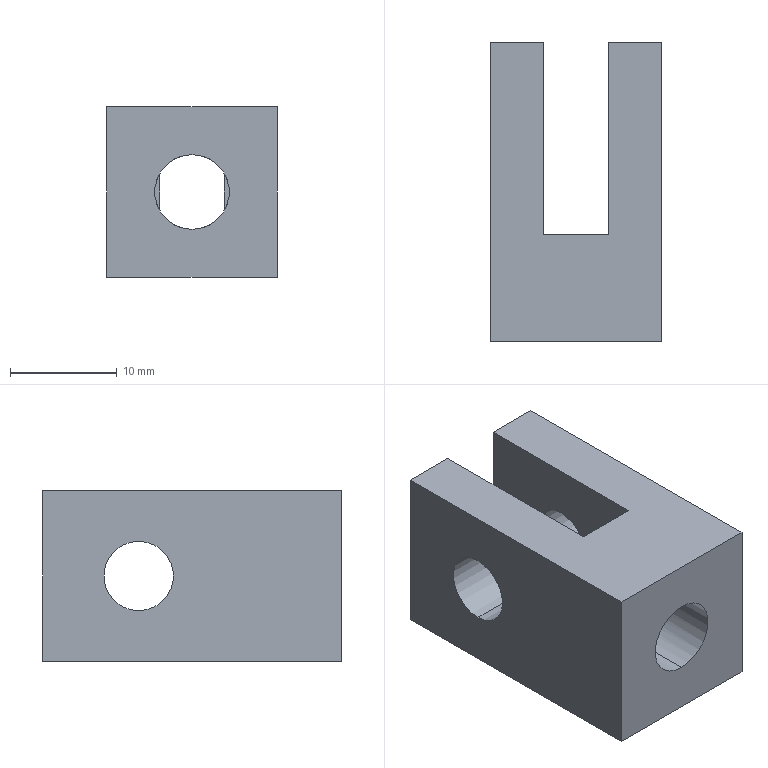Part | STEP file | BU-C05-1 | 1 solid | 19 faces | box 16 x 28 x 16 mm | volume 4723 mm3 | plane 13 | cylinder 6 | commonest cylinder face diameters 6.5 x4 7 x2
STEP:
#1=CARTESIAN_POINT('',(0.,0.,0.));
#2=DIRECTION('',(0.,0.,1.));
#3=DIRECTION('',(1.,0.,0.));
#4=AXIS2_PLACEMENT_3D('',#1,#2,#3);
#5=CARTESIAN_POINT('',(-3.,19.,11.25));
#6=VERTEX_POINT('',#5);
#7=CARTESIAN_POINT('',(-8.,19.,11.25));
#8=VERTEX_POINT('',#7);
#9=CARTESIAN_POINT('',(-8.,19.,11.25));
#10=DIRECTION('',(-1.,0.,0.));
#11=VECTOR('',#10,1.);
#12=LINE('',#9,#11);
#13=CARTESIAN_POINT('',(-8.,19.,8.));
#14=DIRECTION('',(-1.,0.,0.));
#15=DIRECTION('',(0.,0.,1.));
#16=AXIS2_PLACEMENT_3D('',#13,#14,#15);
#17=CYLINDRICAL_SURFACE('',#16,3.25);
#18=CARTESIAN_POINT('',(6.283,0.));
#19=DIRECTION('',(0.,1.));
#20=VECTOR('',#19,1.);
#21=LINE('',#18,#20);
#22=(GEOMETRIC_REPRESENTATION_CONTEXT(2)PARAMETRIC_REPRESENTATION_CONTEXT()REPRESENTATION_CONTEXT('',''));
#23=DEFINITIONAL_REPRESENTATION('',(#21),#22);
#24=PCURVE('',#17,#23);
#25=CARTESIAN_POINT('',(-8.,19.,8.));
#26=DIRECTION('',(-1.,0.,0.));
#27=DIRECTION('',(0.,0.,1.));
#28=AXIS2_PLACEMENT_3D('',#25,#26,#27);
#29=CYLINDRICAL_SURFACE('',#28,3.25);
#30=CARTESIAN_POINT('',(0.,0.));
#31=DIRECTION('',(0.,1.));
#32=VECTOR('',#31,1.);
#33=LINE('',#30,#32);
#34=(GEOMETRIC_REPRESENTATION_CONTEXT(2)PARAMETRIC_REPRESENTATION_CONTEXT()REPRESENTATION_CONTEXT('',''));
#35=DEFINITIONAL_REPRESENTATION('',(#33),#34);
#36=PCURVE('',#29,#35);
#37=SURFACE_CURVE('',#12,(#24,#36),.PCURVE_S1.);
#38=EDGE_CURVE('',#6,#8,#37,.T.);
#39=ORIENTED_EDGE('',*,*,#38,.T.);
#40=CARTESIAN_POINT('',(-8.,19.,4.75));
#41=VERTEX_POINT('',#40);
#42=CARTESIAN_POINT('',(-8.,19.,8.));
#43=DIRECTION('',(-1.,0.,0.));
#44=DIRECTION('',(0.,0.,1.));
#45=AXIS2_PLACEMENT_3D('',#42,#43,#44);
#46=CIRCLE('',#45,3.25);
#47=CARTESIAN_POINT('',(0.,0.));
#48=DIRECTION('',(1.,0.));
#49=VECTOR('',#48,1.);
#50=LINE('',#47,#49);
#51=(GEOMETRIC_REPRESENTATION_CONTEXT(2)PARAMETRIC_REPRESENTATION_CONTEXT()REPRESENTATION_CONTEXT('',''));
#52=DEFINITIONAL_REPRESENTATION('',(#50),#51);
#53=PCURVE('',#17,#52);
#54=CARTESIAN_POINT('',(-8.,0.,16.));
#55=DIRECTION('',(1.,0.,0.));
#56=DIRECTION('',(0.,0.,-1.));
#57=AXIS2_PLACEMENT_3D('',#54,#55,#56);
#58=PLANE('',#57);
#59=CARTESIAN_POINT('',(4.75,19.));
#60=CARTESIAN_POINT('',(4.75,24.629));
#61=CARTESIAN_POINT('',(9.625,21.815));
#62=CARTESIAN_POINT('',(14.5,19.));
#63=CARTESIAN_POINT('',(9.625,16.185));
#64=CARTESIAN_POINT('',(4.75,13.371));
#65=CARTESIAN_POINT('',(4.75,19.));
#66=(BOUNDED_CURVE()B_SPLINE_CURVE(2,(#59,#60,#61,#62,#63,#64,#65),.UNSPECIFIED.,.T.,.F.)B_SPLINE_CURVE_WITH_KNOTS((1,2,2,2,2,1),(-2.094,0.,2.094,4.189,6.283,8.378),.UNSPECIFIED.)CURVE()GEOMETRIC_REPRESENTATION_ITEM()RATIONAL_B_SPLINE_CURVE((1.,0.5,1.,0.5,1.,0.5,1.))REPRESENTATION_ITEM(''));
#67=(GEOMETRIC_REPRESENTATION_CONTEXT(2)PARAMETRIC_REPRESENTATION_CONTEXT()REPRESENTATION_CONTEXT('',''));
#68=DEFINITIONAL_REPRESENTATION('',(#66),#67);
#69=PCURVE('',#58,#68);
#70=SURFACE_CURVE('',#46,(#53,#69),.PCURVE_S1.);
#71=EDGE_CURVE('',#41,#8,#70,.T.);
#72=ORIENTED_EDGE('',*,*,#71,.F.);
#73=CARTESIAN_POINT('',(-3.,19.,4.75));
#74=VERTEX_POINT('',#73);
#75=CARTESIAN_POINT('',(-8.,19.,4.75));
#76=DIRECTION('',(-1.,0.,0.));
#77=VECTOR('',#76,1.);
#78=LINE('',#75,#77);
#79=CARTESIAN_POINT('',(3.142,0.));
#80=DIRECTION('',(0.,1.));
#81=VECTOR('',#80,1.);
#82=LINE('',#79,#81);
#83=(GEOMETRIC_REPRESENTATION_CONTEXT(2)PARAMETRIC_REPRESENTATION_CONTEXT()REPRESENTATION_CONTEXT('',''));
#84=DEFINITIONAL_REPRESENTATION('',(#82),#83);
#85=PCURVE('',#17,#84);
#86=CARTESIAN_POINT('',(3.142,0.));
#87=DIRECTION('',(0.,1.));
#88=VECTOR('',#87,1.);
#89=LINE('',#86,#88);
#90=(GEOMETRIC_REPRESENTATION_CONTEXT(2)PARAMETRIC_REPRESENTATION_CONTEXT()REPRESENTATION_CONTEXT('',''));
#91=DEFINITIONAL_REPRESENTATION('',(#89),#90);
#92=PCURVE('',#29,#91);
#93=SURFACE_CURVE('',#78,(#85,#92),.PCURVE_S1.);
#94=EDGE_CURVE('',#74,#41,#93,.T.);
#95=ORIENTED_EDGE('',*,*,#94,.F.);
#96=CARTESIAN_POINT('',(-3.,19.,8.));
#97=DIRECTION('',(-1.,0.,0.));
#98=DIRECTION('',(0.,0.,1.));
#99=AXIS2_PLACEMENT_3D('',#96,#97,#98);
#100=CIRCLE('',#99,3.25);
#101=CARTESIAN_POINT('',(0.,-5.));
#102=DIRECTION('',(1.,0.));
#103=VECTOR('',#102,1.);
#104=LINE('',#101,#103);
#105=(GEOMETRIC_REPRESENTATION_CONTEXT(2)PARAMETRIC_REPRESENTATION_CONTEXT()REPRESENTATION_CONTEXT('',''));
#106=DEFINITIONAL_REPRESENTATION('',(#104),#105);
#107=PCURVE('',#17,#106);
#108=CARTESIAN_POINT('',(-3.,10.,16.));
#109=DIRECTION('',(-1.,0.,0.));
#110=DIRECTION('',(0.,0.,1.));
#111=AXIS2_PLACEMENT_3D('',#108,#109,#110);
#112=PLANE('',#111);
#113=CARTESIAN_POINT('',(-8.,9.));
#114=DIRECTION('',(1.,0.));
#115=AXIS2_PLACEMENT_2D('',#113,#114);
#116=CIRCLE('',#115,3.25);
#117=(GEOMETRIC_REPRESENTATION_CONTEXT(2)PARAMETRIC_REPRESENTATION_CONTEXT()REPRESENTATION_CONTEXT('',''));
#118=DEFINITIONAL_REPRESENTATION('',(#116),#117);
#119=PCURVE('',#112,#118);
#120=SURFACE_CURVE('',#100,(#107,#119),.PCURVE_S1.);
#121=EDGE_CURVE('',#74,#6,#120,.T.);
#122=ORIENTED_EDGE('',*,*,#121,.T.);
#123=EDGE_LOOP('',(#39,#72,#95,#122));
#124=FACE_BOUND('',#123,.F.);
#125=ADVANCED_FACE('',(#124),#17,.F.);
#126=CARTESIAN_POINT('',(8.,19.,11.25));
#127=VERTEX_POINT('',#126);
#128=CARTESIAN_POINT('',(3.,19.,11.25));
#129=VERTEX_POINT('',#128);
#130=CARTESIAN_POINT('',(-8.,19.,11.25));
#131=DIRECTION('',(-1.,0.,0.));
#132=VECTOR('',#131,1.);
#133=LINE('',#130,#132);
#134=CARTESIAN_POINT('',(-8.,19.,8.));
#135=DIRECTION('',(-1.,0.,0.));
#136=DIRECTION('',(0.,0.,1.));
#137=AXIS2_PLACEMENT_3D('',#134,#135,#136);
#138=CYLINDRICAL_SURFACE('',#137,3.25);
#139=CARTESIAN_POINT('',(6.283,0.));
#140=DIRECTION('',(0.,1.));
#141=VECTOR('',#140,1.);
#142=LINE('',#139,#141);
#143=(GEOMETRIC_REPRESENTATION_CONTEXT(2)PARAMETRIC_REPRESENTATION_CONTEXT()REPRESENTATION_CONTEXT('',''));
#144=DEFINITIONAL_REPRESENTATION('',(#142),#143);
#145=PCURVE('',#138,#144);
#146=CARTESIAN_POINT('',(-8.,19.,8.));
#147=DIRECTION('',(-1.,0.,0.));
#148=DIRECTION('',(0.,0.,1.));
#149=AXIS2_PLACEMENT_3D('',#146,#147,#148);
#150=CYLINDRICAL_SURFACE('',#149,3.25);
#151=CARTESIAN_POINT('',(0.,0.));
#152=DIRECTION('',(0.,1.));
#153=VECTOR('',#152,1.);
#154=LINE('',#151,#153);
#155=(GEOMETRIC_REPRESENTATION_CONTEXT(2)PARAMETRIC_REPRESENTATION_CONTEXT()REPRESENTATION_CONTEXT('',''));
#156=DEFINITIONAL_REPRESENTATION('',(#154),#155);
#157=PCURVE('',#150,#156);
#158=SURFACE_CURVE('',#133,(#145,#157),.PCURVE_S1.);
#159=EDGE_CURVE('',#127,#129,#158,.T.);
#160=ORIENTED_EDGE('',*,*,#159,.T.);
#161=CARTESIAN_POINT('',(3.,19.,4.75));
#162=VERTEX_POINT('',#161);
#163=CARTESIAN_POINT('',(3.,19.,8.));
#164=DIRECTION('',(1.,0.,0.));
#165=DIRECTION('',(0.,0.,-1.));
#166=AXIS2_PLACEMENT_3D('',#163,#164,#165);
#167=CIRCLE('',#166,3.25);
#168=CARTESIAN_POINT('',(9.425,-11.));
#169=DIRECTION('',(-1.,0.));
#170=VECTOR('',#169,1.);
#171=LINE('',#168,#170);
#172=(GEOMETRIC_REPRESENTATION_CONTEXT(2)PARAMETRIC_REPRESENTATION_CONTEXT()REPRESENTATION_CONTEXT('',''));
#173=DEFINITIONAL_REPRESENTATION('',(#171),#172);
#174=PCURVE('',#138,#173);
#175=CARTESIAN_POINT('',(3.,10.,16.));
#176=DIRECTION('',(1.,0.,0.));
#177=DIRECTION('',(0.,0.,-1.));
#178=AXIS2_PLACEMENT_3D('',#175,#176,#177);
#179=PLANE('',#178);
#180=CARTESIAN_POINT('',(8.,9.));
#181=DIRECTION('',(1.,0.));
#182=AXIS2_PLACEMENT_2D('',#180,#181);
#183=CIRCLE('',#182,3.25);
#184=(GEOMETRIC_REPRESENTATION_CONTEXT(2)PARAMETRIC_REPRESENTATION_CONTEXT()REPRESENTATION_CONTEXT('',''));
#185=DEFINITIONAL_REPRESENTATION('',(#183),#184);
#186=PCURVE('',#179,#185);
#187=SURFACE_CURVE('',#167,(#174,#186),.PCURVE_S1.);
#188=EDGE_CURVE('',#129,#162,#187,.T.);
#189=ORIENTED_EDGE('',*,*,#188,.T.);
#190=CARTESIAN_POINT('',(8.,19.,4.75));
#191=VERTEX_POINT('',#190);
#192=CARTESIAN_POINT('',(-8.,19.,4.75));
#193=DIRECTION('',(-1.,0.,0.));
#194=VECTOR('',#193,1.);
#195=LINE('',#192,#194);
#196=CARTESIAN_POINT('',(3.142,0.));
#197=DIRECTION('',(0.,1.));
#198=VECTOR('',#197,1.);
#199=LINE('',#196,#198);
#200=(GEOMETRIC_REPRESENTATION_CONTEXT(2)PARAMETRIC_REPRESENTATION_CONTEXT()REPRESENTATION_CONTEXT('',''));
#201=DEFINITIONAL_REPRESENTATION('',(#199),#200);
#202=PCURVE('',#138,#201);
#203=CARTESIAN_POINT('',(3.142,0.));
#204=DIRECTION('',(0.,1.));
#205=VECTOR('',#204,1.);
#206=LINE('',#203,#205);
#207=(GEOMETRIC_REPRESENTATION_CONTEXT(2)PARAMETRIC_REPRESENTATION_CONTEXT()REPRESENTATION_CONTEXT('',''));
#208=DEFINITIONAL_REPRESENTATION('',(#206),#207);
#209=PCURVE('',#150,#208);
#210=SURFACE_CURVE('',#195,(#202,#209),.PCURVE_S1.);
#211=EDGE_CURVE('',#191,#162,#210,.T.);
#212=ORIENTED_EDGE('',*,*,#211,.F.);
#213=CARTESIAN_POINT('',(8.,19.,8.));
#214=DIRECTION('',(-1.,0.,0.));
#215=DIRECTION('',(0.,0.,1.));
#216=AXIS2_PLACEMENT_3D('',#213,#214,#215);
#217=CIRCLE('',#216,3.25);
#218=CARTESIAN_POINT('',(0.,-16.));
#219=DIRECTION('',(1.,0.));
#220=VECTOR('',#219,1.);
#221=LINE('',#218,#220);
#222=(GEOMETRIC_REPRESENTATION_CONTEXT(2)PARAMETRIC_REPRESENTATION_CONTEXT()REPRESENTATION_CONTEXT('',''));
#223=DEFINITIONAL_REPRESENTATION('',(#221),#222);
#224=PCURVE('',#138,#223);
#225=CARTESIAN_POINT('',(8.,0.,16.));
#226=DIRECTION('',(-1.,0.,0.));
#227=DIRECTION('',(0.,0.,1.));
#228=AXIS2_PLACEMENT_3D('',#225,#226,#227);
#229=PLANE('',#228);
#230=CARTESIAN_POINT('',(-8.,19.));
#231=DIRECTION('',(1.,0.));
#232=AXIS2_PLACEMENT_2D('',#230,#231);
#233=CIRCLE('',#232,3.25);
#234=(GEOMETRIC_REPRESENTATION_CONTEXT(2)PARAMETRIC_REPRESENTATION_CONTEXT()REPRESENTATION_CONTEXT('',''));
#235=DEFINITIONAL_REPRESENTATION('',(#233),#234);
#236=PCURVE('',#229,#235);
#237=SURFACE_CURVE('',#217,(#224,#236),.PCURVE_S1.);
#238=EDGE_CURVE('',#191,#127,#237,.T.);
#239=ORIENTED_EDGE('',*,*,#238,.T.);
#240=EDGE_LOOP('',(#160,#189,#212,#239));
#241=FACE_BOUND('',#240,.F.);
#242=ADVANCED_FACE('',(#241),#138,.F.);
#243=CARTESIAN_POINT('',(-3.,10.,6.197));
#244=VERTEX_POINT('',#243);
#245=CARTESIAN_POINT('',(-3.,10.,9.803));
#246=VERTEX_POINT('',#245);
#247=CARTESIAN_POINT('',(0.,10.,8.));
#248=DIRECTION('',(0.,1.,0.));
#249=DIRECTION('',(0.,0.,-1.));
#250=AXIS2_PLACEMENT_3D('',#247,#248,#249);
#251=CIRCLE('',#250,3.5);
#252=CARTESIAN_POINT('',(0.,0.,8.));
#253=DIRECTION('',(0.,-1.,0.));
#254=DIRECTION('',(0.,0.,-1.));
#255=AXIS2_PLACEMENT_3D('',#252,#253,#254);
#256=CYLINDRICAL_SURFACE('',#255,3.5);
#257=CARTESIAN_POINT('',(6.283,-10.));
#258=DIRECTION('',(-1.,0.));
#259=VECTOR('',#258,1.);
#260=LINE('',#257,#259);
#261=(GEOMETRIC_REPRESENTATION_CONTEXT(2)PARAMETRIC_REPRESENTATION_CONTEXT()REPRESENTATION_CONTEXT('',''));
#262=DEFINITIONAL_REPRESENTATION('',(#260),#261);
#263=PCURVE('',#256,#262);
#264=CARTESIAN_POINT('',(-3.,10.,16.));
#265=DIRECTION('',(0.,-1.,0.));
#266=DIRECTION('',(0.,0.,-1.));
#267=AXIS2_PLACEMENT_3D('',#264,#265,#266);
#268=PLANE('',#267);
#269=CARTESIAN_POINT('',(11.5,3.));
#270=CARTESIAN_POINT('',(11.5,-3.062));
#271=CARTESIAN_POINT('',(6.25,-0.03109));
#272=CARTESIAN_POINT('',(1.,3.));
#273=CARTESIAN_POINT('',(6.25,6.031));
#274=CARTESIAN_POINT('',(11.5,9.062));
#275=CARTESIAN_POINT('',(11.5,3.));
#276=(BOUNDED_CURVE()B_SPLINE_CURVE(2,(#269,#270,#271,#272,#273,#274,#275),.UNSPECIFIED.,.T.,.F.)B_SPLINE_CURVE_WITH_KNOTS((1,2,2,2,2,1),(-2.094,0.,2.094,4.189,6.283,8.378),.UNSPECIFIED.)CURVE()GEOMETRIC_REPRESENTATION_ITEM()RATIONAL_B_SPLINE_CURVE((1.,0.5,1.,0.5,1.,0.5,1.))REPRESENTATION_ITEM(''));
#277=(GEOMETRIC_REPRESENTATION_CONTEXT(2)PARAMETRIC_REPRESENTATION_CONTEXT()REPRESENTATION_CONTEXT('',''));
#278=DEFINITIONAL_REPRESENTATION('',(#276),#277);
#279=PCURVE('',#268,#278);
#280=SURFACE_CURVE('',#251,(#263,#279),.PCURVE_S1.);
#281=EDGE_CURVE('',#244,#246,#280,.T.);
#282=ORIENTED_EDGE('',*,*,#281,.F.);
#283=CARTESIAN_POINT('',(0.,10.,4.5));
#284=VERTEX_POINT('',#283);
#285=CARTESIAN_POINT('',(0.,10.,8.));
#286=DIRECTION('',(0.,1.,0.));
#287=DIRECTION('',(0.,0.,-1.));
#288=AXIS2_PLACEMENT_3D('',#285,#286,#287);
#289=CIRCLE('',#288,3.5);
#290=CARTESIAN_POINT('',(6.283,-10.));
#291=DIRECTION('',(-1.,0.));
#292=VECTOR('',#291,1.);
#293=LINE('',#290,#292);
#294=(GEOMETRIC_REPRESENTATION_CONTEXT(2)PARAMETRIC_REPRESENTATION_CONTEXT()REPRESENTATION_CONTEXT('',''));
#295=DEFINITIONAL_REPRESENTATION('',(#293),#294);
#296=PCURVE('',#256,#295);
#297=CARTESIAN_POINT('',(-3.,10.,16.));
#298=DIRECTION('',(0.,-1.,0.));
#299=DIRECTION('',(0.,0.,-1.));
#300=AXIS2_PLACEMENT_3D('',#297,#298,#299);
#301=PLANE('',#300);
#302=CARTESIAN_POINT('',(11.5,3.));
#303=CARTESIAN_POINT('',(11.5,-3.062));
#304=CARTESIAN_POINT('',(6.25,-0.03109));
#305=CARTESIAN_POINT('',(1.,3.));
#306=CARTESIAN_POINT('',(6.25,6.031));
#307=CARTESIAN_POINT('',(11.5,9.062));
#308=CARTESIAN_POINT('',(11.5,3.));
#309=(BOUNDED_CURVE()B_SPLINE_CURVE(2,(#302,#303,#304,#305,#306,#307,#308),.UNSPECIFIED.,.T.,.F.)B_SPLINE_CURVE_WITH_KNOTS((1,2,2,2,2,1),(-2.094,0.,2.094,4.189,6.283,8.378),.UNSPECIFIED.)CURVE()GEOMETRIC_REPRESENTATION_ITEM()RATIONAL_B_SPLINE_CURVE((1.,0.5,1.,0.5,1.,0.5,1.))REPRESENTATION_ITEM(''));
#310=(GEOMETRIC_REPRESENTATION_CONTEXT(2)PARAMETRIC_REPRESENTATION_CONTEXT()REPRESENTATION_CONTEXT('',''));
#311=DEFINITIONAL_REPRESENTATION('',(#309),#310);
#312=PCURVE('',#301,#311);
#313=SURFACE_CURVE('',#289,(#296,#312),.PCURVE_S1.);
#314=EDGE_CURVE('',#284,#244,#313,.T.);
#315=ORIENTED_EDGE('',*,*,#314,.F.);
#316=CARTESIAN_POINT('',(0.,0.,4.5));
#317=VERTEX_POINT('',#316);
#318=CARTESIAN_POINT('',(0.,0.,4.5));
#319=DIRECTION('',(0.,-1.,0.));
#320=VECTOR('',#319,1.);
#321=LINE('',#318,#320);
#322=CARTESIAN_POINT('',(6.283,0.));
#323=DIRECTION('',(0.,1.));
#324=VECTOR('',#323,1.);
#325=LINE('',#322,#324);
#326=(GEOMETRIC_REPRESENTATION_CONTEXT(2)PARAMETRIC_REPRESENTATION_CONTEXT()REPRESENTATION_CONTEXT('',''));
#327=DEFINITIONAL_REPRESENTATION('',(#325),#326);
#328=PCURVE('',#256,#327);
#329=CARTESIAN_POINT('',(0.,0.,8.));
#330=DIRECTION('',(0.,-1.,0.));
#331=DIRECTION('',(0.,0.,-1.));
#332=AXIS2_PLACEMENT_3D('',#329,#330,#331);
#333=CYLINDRICAL_SURFACE('',#332,3.5);
#334=CARTESIAN_POINT('',(0.,0.));
#335=DIRECTION('',(0.,1.));
#336=VECTOR('',#335,1.);
#337=LINE('',#334,#336);
#338=(GEOMETRIC_REPRESENTATION_CONTEXT(2)PARAMETRIC_REPRESENTATION_CONTEXT()REPRESENTATION_CONTEXT('',''));
#339=DEFINITIONAL_REPRESENTATION('',(#337),#338);
#340=PCURVE('',#333,#339);
#341=SURFACE_CURVE('',#321,(#328,#340),.PCURVE_S1.);
#342=EDGE_CURVE('',#284,#317,#341,.T.);
#343=ORIENTED_EDGE('',*,*,#342,.T.);
#344=CARTESIAN_POINT('',(0.,0.,11.5));
#345=VERTEX_POINT('',#344);
#346=CARTESIAN_POINT('',(0.,0.,8.));
#347=DIRECTION('',(0.,-1.,0.));
#348=DIRECTION('',(0.,0.,-1.));
#349=AXIS2_PLACEMENT_3D('',#346,#347,#348);
#350=CIRCLE('',#349,3.5);
#351=CARTESIAN_POINT('',(0.,0.));
#352=DIRECTION('',(1.,0.));
#353=VECTOR('',#352,1.);
#354=LINE('',#351,#353);
#355=(GEOMETRIC_REPRESENTATION_CONTEXT(2)PARAMETRIC_REPRESENTATION_CONTEXT()REPRESENTATION_CONTEXT('',''));
#356=DEFINITIONAL_REPRESENTATION('',(#354),#355);
#357=PCURVE('',#256,#356);
#358=CARTESIAN_POINT('',(-8.,0.,16.));
#359=DIRECTION('',(0.,1.,0.));
#360=DIRECTION('',(0.,0.,1.));
#361=AXIS2_PLACEMENT_3D('',#358,#359,#360);
#362=PLANE('',#361);
#363=CARTESIAN_POINT('',(-11.5,8.));
#364=CARTESIAN_POINT('',(-11.5,14.062));
#365=CARTESIAN_POINT('',(-6.25,11.031));
#366=CARTESIAN_POINT('',(-1.,8.));
#367=CARTESIAN_POINT('',(-6.25,4.969));
#368=CARTESIAN_POINT('',(-11.5,1.938));
#369=CARTESIAN_POINT('',(-11.5,8.));
#370=(BOUNDED_CURVE()B_SPLINE_CURVE(2,(#363,#364,#365,#366,#367,#368,#369),.UNSPECIFIED.,.T.,.F.)B_SPLINE_CURVE_WITH_KNOTS((1,2,2,2,2,1),(-2.094,0.,2.094,4.189,6.283,8.378),.UNSPECIFIED.)CURVE()GEOMETRIC_REPRESENTATION_ITEM()RATIONAL_B_SPLINE_CURVE((1.,0.5,1.,0.5,1.,0.5,1.))REPRESENTATION_ITEM(''));
#371=(GEOMETRIC_REPRESENTATION_CONTEXT(2)PARAMETRIC_REPRESENTATION_CONTEXT()REPRESENTATION_CONTEXT('',''));
#372=DEFINITIONAL_REPRESENTATION('',(#370),#371);
#373=PCURVE('',#362,#372);
#374=SURFACE_CURVE('',#350,(#357,#373),.PCURVE_S1.);
#375=EDGE_CURVE('',#345,#317,#374,.T.);
#376=ORIENTED_EDGE('',*,*,#375,.F.);
#377=CARTESIAN_POINT('',(0.,10.,11.5));
#378=VERTEX_POINT('',#377);
#379=CARTESIAN_POINT('',(0.,0.,11.5));
#380=DIRECTION('',(0.,-1.,0.));
#381=VECTOR('',#380,1.);
#382=LINE('',#379,#381);
#383=CARTESIAN_POINT('',(3.142,0.));
#384=DIRECTION('',(0.,1.));
#385=VECTOR('',#384,1.);
#386=LINE('',#383,#385);
#387=(GEOMETRIC_REPRESENTATION_CONTEXT(2)PARAMETRIC_REPRESENTATION_CONTEXT()REPRESENTATION_CONTEXT('',''));
#388=DEFINITIONAL_REPRESENTATION('',(#386),#387);
#389=PCURVE('',#256,#388);
#390=CARTESIAN_POINT('',(3.142,0.));
#391=DIRECTION('',(0.,1.));
#392=VECTOR('',#391,1.);
#393=LINE('',#390,#392);
#394=(GEOMETRIC_REPRESENTATION_CONTEXT(2)PARAMETRIC_REPRESENTATION_CONTEXT()REPRESENTATION_CONTEXT('',''));
#395=DEFINITIONAL_REPRESENTATION('',(#393),#394);
#396=PCURVE('',#333,#395);
#397=SURFACE_CURVE('',#382,(#389,#396),.PCURVE_S1.);
#398=EDGE_CURVE('',#378,#345,#397,.T.);
#399=ORIENTED_EDGE('',*,*,#398,.F.);
#400=CARTESIAN_POINT('',(0.,10.,8.));
#401=DIRECTION('',(0.,1.,0.));
#402=DIRECTION('',(0.,0.,-1.));
#403=AXIS2_PLACEMENT_3D('',#400,#401,#402);
#404=CIRCLE('',#403,3.5);
#405=CARTESIAN_POINT('',(6.283,-10.));
#406=DIRECTION('',(-1.,0.));
#407=VECTOR('',#406,1.);
#408=LINE('',#405,#407);
#409=(GEOMETRIC_REPRESENTATION_CONTEXT(2)PARAMETRIC_REPRESENTATION_CONTEXT()REPRESENTATION_CONTEXT('',''));
#410=DEFINITIONAL_REPRESENTATION('',(#408),#409);
#411=PCURVE('',#256,#410);
#412=CARTESIAN_POINT('',(-3.,10.,16.));
#413=DIRECTION('',(0.,-1.,0.));
#414=DIRECTION('',(0.,0.,-1.));
#415=AXIS2_PLACEMENT_3D('',#412,#413,#414);
#416=PLANE('',#415);
#417=CARTESIAN_POINT('',(11.5,3.));
#418=CARTESIAN_POINT('',(11.5,-3.062));
#419=CARTESIAN_POINT('',(6.25,-0.03109));
#420=CARTESIAN_POINT('',(1.,3.));
#421=CARTESIAN_POINT('',(6.25,6.031));
#422=CARTESIAN_POINT('',(11.5,9.062));
#423=CARTESIAN_POINT('',(11.5,3.));
#424=(BOUNDED_CURVE()B_SPLINE_CURVE(2,(#417,#418,#419,#420,#421,#422,#423),.UNSPECIFIED.,.T.,.F.)B_SPLINE_CURVE_WITH_KNOTS((1,2,2,2,2,1),(-2.094,0.,2.094,4.189,6.283,8.378),.UNSPECIFIED.)CURVE()GEOMETRIC_REPRESENTATION_ITEM()RATIONAL_B_SPLINE_CURVE((1.,0.5,1.,0.5,1.,0.5,1.))REPRESENTATION_ITEM(''));
#425=(GEOMETRIC_REPRESENTATION_CONTEXT(2)PARAMETRIC_REPRESENTATION_CONTEXT()REPRESENTATION_CONTEXT('',''));
#426=DEFINITIONAL_REPRESENTATION('',(#424),#425);
#427=PCURVE('',#416,#426);
#428=SURFACE_CURVE('',#404,(#411,#427),.PCURVE_S1.);
#429=EDGE_CURVE('',#246,#378,#428,.T.);
#430=ORIENTED_EDGE('',*,*,#429,.F.);
#431=EDGE_LOOP('',(#282,#315,#343,#376,#399,#430));
#432=FACE_BOUND('',#431,.F.);
#433=ADVANCED_FACE('',(#432),#256,.F.);
#434=ORIENTED_EDGE('',*,*,#429,.F.);
#435=CARTESIAN_POINT('',(-3.,10.,16.));
#436=VERTEX_POINT('',#435);
#437=CARTESIAN_POINT('',(-3.,10.,16.));
#438=DIRECTION('',(0.,0.,-1.));
#439=VECTOR('',#438,1.);
#440=LINE('',#437,#439);
#441=CARTESIAN_POINT('',(0.,0.));
#442=DIRECTION('',(1.,0.));
#443=VECTOR('',#442,1.);
#444=LINE('',#441,#443);
#445=(GEOMETRIC_REPRESENTATION_CONTEXT(2)PARAMETRIC_REPRESENTATION_CONTEXT()REPRESENTATION_CONTEXT('',''));
#446=DEFINITIONAL_REPRESENTATION('',(#444),#445);
#447=PCURVE('',#416,#446);
#448=CARTESIAN_POINT('',(0.,0.));
#449=DIRECTION('',(-1.,0.));
#450=VECTOR('',#449,1.);
#451=LINE('',#448,#450);
#452=(GEOMETRIC_REPRESENTATION_CONTEXT(2)PARAMETRIC_REPRESENTATION_CONTEXT()REPRESENTATION_CONTEXT('',''));
#453=DEFINITIONAL_REPRESENTATION('',(#451),#452);
#454=PCURVE('',#112,#453);
#455=SURFACE_CURVE('',#440,(#447,#454),.PCURVE_S1.);
#456=EDGE_CURVE('',#436,#246,#455,.T.);
#457=ORIENTED_EDGE('',*,*,#456,.F.);
#458=CARTESIAN_POINT('',(3.,10.,16.));
#459=VERTEX_POINT('',#458);
#460=CARTESIAN_POINT('',(-3.,10.,16.));
#461=DIRECTION('',(-1.,0.,0.));
#462=VECTOR('',#461,1.);
#463=LINE('',#460,#462);
#464=CARTESIAN_POINT('',(0.,0.));
#465=DIRECTION('',(0.,-1.));
#466=VECTOR('',#465,1.);
#467=LINE('',#464,#466);
#468=(GEOMETRIC_REPRESENTATION_CONTEXT(2)PARAMETRIC_REPRESENTATION_CONTEXT()REPRESENTATION_CONTEXT('',''));
#469=DEFINITIONAL_REPRESENTATION('',(#467),#468);
#470=PCURVE('',#416,#469);
#471=CARTESIAN_POINT('',(3.,10.,16.));
#472=DIRECTION('',(0.,0.,1.));
#473=DIRECTION('',(1.,0.,0.));
#474=AXIS2_PLACEMENT_3D('',#471,#472,#473);
#475=PLANE('',#474);
#476=CARTESIAN_POINT('',(-6.,0.));
#477=DIRECTION('',(-1.,0.));
#478=VECTOR('',#477,1.);
#479=LINE('',#476,#478);
#480=(GEOMETRIC_REPRESENTATION_CONTEXT(2)PARAMETRIC_REPRESENTATION_CONTEXT()REPRESENTATION_CONTEXT('',''));
#481=DEFINITIONAL_REPRESENTATION('',(#479),#480);
#482=PCURVE('',#475,#481);
#483=SURFACE_CURVE('',#463,(#470,#482),.PCURVE_S1.);
#484=EDGE_CURVE('',#459,#436,#483,.T.);
#485=ORIENTED_EDGE('',*,*,#484,.F.);
#486=CARTESIAN_POINT('',(3.,10.,9.803));
#487=VERTEX_POINT('',#486);
#488=CARTESIAN_POINT('',(3.,10.,16.));
#489=DIRECTION('',(0.,0.,-1.));
#490=VECTOR('',#489,1.);
#491=LINE('',#488,#490);
#492=CARTESIAN_POINT('',(0.,6.));
#493=DIRECTION('',(1.,0.));
#494=VECTOR('',#493,1.);
#495=LINE('',#492,#494);
#496=(GEOMETRIC_REPRESENTATION_CONTEXT(2)PARAMETRIC_REPRESENTATION_CONTEXT()REPRESENTATION_CONTEXT('',''));
#497=DEFINITIONAL_REPRESENTATION('',(#495),#496);
#498=PCURVE('',#416,#497);
#499=CARTESIAN_POINT('',(0.,0.));
#500=DIRECTION('',(1.,0.));
#501=VECTOR('',#500,1.);
#502=LINE('',#499,#501);
#503=(GEOMETRIC_REPRESENTATION_CONTEXT(2)PARAMETRIC_REPRESENTATION_CONTEXT()REPRESENTATION_CONTEXT('',''));
#504=DEFINITIONAL_REPRESENTATION('',(#502),#503);
#505=PCURVE('',#179,#504);
#506=SURFACE_CURVE('',#491,(#498,#505),.PCURVE_S1.);
#507=EDGE_CURVE('',#459,#487,#506,.T.);
#508=ORIENTED_EDGE('',*,*,#507,.T.);
#509=CARTESIAN_POINT('',(0.,10.,8.));
#510=DIRECTION('',(0.,1.,0.));
#511=DIRECTION('',(0.,0.,-1.));
#512=AXIS2_PLACEMENT_3D('',#509,#510,#511);
#513=CIRCLE('',#512,3.5);
#514=CARTESIAN_POINT('',(11.5,3.));
#515=CARTESIAN_POINT('',(11.5,-3.062));
#516=CARTESIAN_POINT('',(6.25,-0.03109));
#517=CARTESIAN_POINT('',(1.,3.));
#518=CARTESIAN_POINT('',(6.25,6.031));
#519=CARTESIAN_POINT('',(11.5,9.062));
#520=CARTESIAN_POINT('',(11.5,3.));
#521=(BOUNDED_CURVE()B_SPLINE_CURVE(2,(#514,#515,#516,#517,#518,#519,#520),.UNSPECIFIED.,.T.,.F.)B_SPLINE_CURVE_WITH_KNOTS((1,2,2,2,2,1),(-2.094,0.,2.094,4.189,6.283,8.378),.UNSPECIFIED.)CURVE()GEOMETRIC_REPRESENTATION_ITEM()RATIONAL_B_SPLINE_CURVE((1.,0.5,1.,0.5,1.,0.5,1.))REPRESENTATION_ITEM(''));
#522=(GEOMETRIC_REPRESENTATION_CONTEXT(2)PARAMETRIC_REPRESENTATION_CONTEXT()REPRESENTATION_CONTEXT('',''));
#523=DEFINITIONAL_REPRESENTATION('',(#521),#522);
#524=PCURVE('',#416,#523);
#525=CARTESIAN_POINT('',(6.283,-10.));
#526=DIRECTION('',(-1.,0.));
#527=VECTOR('',#526,1.);
#528=LINE('',#525,#527);
#529=(GEOMETRIC_REPRESENTATION_CONTEXT(2)PARAMETRIC_REPRESENTATION_CONTEXT()REPRESENTATION_CONTEXT('',''));
#530=DEFINITIONAL_REPRESENTATION('',(#528),#529);
#531=PCURVE('',#333,#530);
#532=SURFACE_CURVE('',#513,(#524,#531),.PCURVE_S1.);
#533=EDGE_CURVE('',#378,#487,#532,.T.);
#534=ORIENTED_EDGE('',*,*,#533,.F.);
#535=EDGE_LOOP('',(#434,#457,#485,#508,#534));
#536=FACE_BOUND('',#535,.T.);
#537=ADVANCED_FACE('',(#536),#416,.F.);
#538=CARTESIAN_POINT('',(3.,10.,6.197));
#539=VERTEX_POINT('',#538);
#540=CARTESIAN_POINT('',(0.,10.,8.));
#541=DIRECTION('',(0.,1.,0.));
#542=DIRECTION('',(0.,0.,-1.));
#543=AXIS2_PLACEMENT_3D('',#540,#541,#542);
#544=CIRCLE('',#543,3.5);
#545=CARTESIAN_POINT('',(11.5,3.));
#546=CARTESIAN_POINT('',(11.5,-3.062));
#547=CARTESIAN_POINT('',(6.25,-0.03109));
#548=CARTESIAN_POINT('',(1.,3.));
#549=CARTESIAN_POINT('',(6.25,6.031));
#550=CARTESIAN_POINT('',(11.5,9.062));
#551=CARTESIAN_POINT('',(11.5,3.));
#552=(BOUNDED_CURVE()B_SPLINE_CURVE(2,(#545,#546,#547,#548,#549,#550,#551),.UNSPECIFIED.,.T.,.F.)B_SPLINE_CURVE_WITH_KNOTS((1,2,2,2,2,1),(-2.094,0.,2.094,4.189,6.283,8.378),.UNSPECIFIED.)CURVE()GEOMETRIC_REPRESENTATION_ITEM()RATIONAL_B_SPLINE_CURVE((1.,0.5,1.,0.5,1.,0.5,1.))REPRESENTATION_ITEM(''));
#553=(GEOMETRIC_REPRESENTATION_CONTEXT(2)PARAMETRIC_REPRESENTATION_CONTEXT()REPRESENTATION_CONTEXT('',''));
#554=DEFINITIONAL_REPRESENTATION('',(#552),#553);
#555=PCURVE('',#301,#554);
#556=CARTESIAN_POINT('',(6.283,-10.));
#557=DIRECTION('',(-1.,0.));
#558=VECTOR('',#557,1.);
#559=LINE('',#556,#558);
#560=(GEOMETRIC_REPRESENTATION_CONTEXT(2)PARAMETRIC_REPRESENTATION_CONTEXT()REPRESENTATION_CONTEXT('',''));
#561=DEFINITIONAL_REPRESENTATION('',(#559),#560);
#562=PCURVE('',#333,#561);
#563=SURFACE_CURVE('',#544,(#555,#562),.PCURVE_S1.);
#564=EDGE_CURVE('',#539,#284,#563,.T.);
#565=ORIENTED_EDGE('',*,*,#564,.F.);
#566=CARTESIAN_POINT('',(3.,10.,0.));
#567=VERTEX_POINT('',#566);
#568=CARTESIAN_POINT('',(3.,10.,16.));
#569=DIRECTION('',(0.,0.,-1.));
#570=VECTOR('',#569,1.);
#571=LINE('',#568,#570);
#572=CARTESIAN_POINT('',(0.,6.));
#573=DIRECTION('',(1.,0.));
#574=VECTOR('',#573,1.);
#575=LINE('',#572,#574);
#576=(GEOMETRIC_REPRESENTATION_CONTEXT(2)PARAMETRIC_REPRESENTATION_CONTEXT()REPRESENTATION_CONTEXT('',''));
#577=DEFINITIONAL_REPRESENTATION('',(#575),#576);
#578=PCURVE('',#301,#577);
#579=CARTESIAN_POINT('',(0.,0.));
#580=DIRECTION('',(1.,0.));
#581=VECTOR('',#580,1.);
#582=LINE('',#579,#581);
#583=(GEOMETRIC_REPRESENTATION_CONTEXT(2)PARAMETRIC_REPRESENTATION_CONTEXT()REPRESENTATION_CONTEXT('',''));
#584=DEFINITIONAL_REPRESENTATION('',(#582),#583);
#585=PCURVE('',#179,#584);
#586=SURFACE_CURVE('',#571,(#578,#585),.PCURVE_S1.);
#587=EDGE_CURVE('',#539,#567,#586,.T.);
#588=ORIENTED_EDGE('',*,*,#587,.T.);
#589=CARTESIAN_POINT('',(-3.,10.,0.));
#590=VERTEX_POINT('',#589);
#591=CARTESIAN_POINT('',(-3.,10.,0.));
#592=DIRECTION('',(-1.,0.,0.));
#593=VECTOR('',#592,1.);
#594=LINE('',#591,#593);
#595=CARTESIAN_POINT('',(16.,0.));
#596=DIRECTION('',(0.,-1.));
#597=VECTOR('',#596,1.);
#598=LINE('',#595,#597);
#599=(GEOMETRIC_REPRESENTATION_CONTEXT(2)PARAMETRIC_REPRESENTATION_CONTEXT()REPRESENTATION_CONTEXT('',''));
#600=DEFINITIONAL_REPRESENTATION('',(#598),#599);
#601=PCURVE('',#301,#600);
#602=CARTESIAN_POINT('',(3.,10.,0.));
#603=DIRECTION('',(0.,0.,1.));
#604=DIRECTION('',(1.,0.,0.));
#605=AXIS2_PLACEMENT_3D('',#602,#603,#604);
#606=PLANE('',#605);
#607=CARTESIAN_POINT('',(-6.,0.));
#608=DIRECTION('',(-1.,0.));
#609=VECTOR('',#608,1.);
#610=LINE('',#607,#609);
#611=(GEOMETRIC_REPRESENTATION_CONTEXT(2)PARAMETRIC_REPRESENTATION_CONTEXT()REPRESENTATION_CONTEXT('',''));
#612=DEFINITIONAL_REPRESENTATION('',(#610),#611);
#613=PCURVE('',#606,#612);
#614=SURFACE_CURVE('',#594,(#601,#613),.PCURVE_S1.);
#615=EDGE_CURVE('',#567,#590,#614,.T.);
#616=ORIENTED_EDGE('',*,*,#615,.T.);
#617=CARTESIAN_POINT('',(-3.,10.,16.));
#618=DIRECTION('',(0.,0.,-1.));
#619=VECTOR('',#618,1.);
#620=LINE('',#617,#619);
#621=CARTESIAN_POINT('',(0.,0.));
#622=DIRECTION('',(1.,0.));
#623=VECTOR('',#622,1.);
#624=LINE('',#621,#623);
#625=(GEOMETRIC_REPRESENTATION_CONTEXT(2)PARAMETRIC_REPRESENTATION_CONTEXT()REPRESENTATION_CONTEXT('',''));
#626=DEFINITIONAL_REPRESENTATION('',(#624),#625);
#627=PCURVE('',#301,#626);
#628=CARTESIAN_POINT('',(0.,0.));
#629=DIRECTION('',(-1.,0.));
#630=VECTOR('',#629,1.);
#631=LINE('',#628,#630);
#632=(GEOMETRIC_REPRESENTATION_CONTEXT(2)PARAMETRIC_REPRESENTATION_CONTEXT()REPRESENTATION_CONTEXT('',''));
#633=DEFINITIONAL_REPRESENTATION('',(#631),#632);
#634=PCURVE('',#112,#633);
#635=SURFACE_CURVE('',#620,(#627,#634),.PCURVE_S1.);
#636=EDGE_CURVE('',#244,#590,#635,.T.);
#637=ORIENTED_EDGE('',*,*,#636,.F.);
#638=ORIENTED_EDGE('',*,*,#314,.F.);
#639=EDGE_LOOP('',(#565,#588,#616,#637,#638));
#640=FACE_BOUND('',#639,.T.);
#641=ADVANCED_FACE('',(#640),#301,.F.);
#642=CARTESIAN_POINT('',(-3.,19.,8.));
#643=DIRECTION('',(-1.,0.,0.));
#644=DIRECTION('',(0.,0.,1.));
#645=AXIS2_PLACEMENT_3D('',#642,#643,#644);
#646=CIRCLE('',#645,3.25);
#647=CARTESIAN_POINT('',(-8.,9.));
#648=DIRECTION('',(1.,0.));
#649=AXIS2_PLACEMENT_2D('',#647,#648);
#650=CIRCLE('',#649,3.25);
#651=(GEOMETRIC_REPRESENTATION_CONTEXT(2)PARAMETRIC_REPRESENTATION_CONTEXT()REPRESENTATION_CONTEXT('',''));
#652=DEFINITIONAL_REPRESENTATION('',(#650),#651);
#653=PCURVE('',#112,#652);
#654=CARTESIAN_POINT('',(0.,-5.));
#655=DIRECTION('',(1.,0.));
#656=VECTOR('',#655,1.);
#657=LINE('',#654,#656);
#658=(GEOMETRIC_REPRESENTATION_CONTEXT(2)PARAMETRIC_REPRESENTATION_CONTEXT()REPRESENTATION_CONTEXT('',''));
#659=DEFINITIONAL_REPRESENTATION('',(#657),#658);
#660=PCURVE('',#29,#659);
#661=SURFACE_CURVE('',#646,(#653,#660),.PCURVE_S1.);
#662=EDGE_CURVE('',#6,#74,#661,.T.);
#663=ORIENTED_EDGE('',*,*,#662,.T.);
#664=ORIENTED_EDGE('',*,*,#121,.T.);
#665=EDGE_LOOP('',(#663,#664));
#666=FACE_BOUND('',#665,.T.);
#667=CARTESIAN_POINT('',(-3.,28.,0.));
#668=VERTEX_POINT('',#667);
#669=CARTESIAN_POINT('',(-3.,10.,0.));
#670=DIRECTION('',(0.,1.,0.));
#671=VECTOR('',#670,1.);
#672=LINE('',#669,#671);
#673=CARTESIAN_POINT('',(-16.,0.));
#674=DIRECTION('',(0.,1.));
#675=VECTOR('',#674,1.);
#676=LINE('',#673,#675);
#677=(GEOMETRIC_REPRESENTATION_CONTEXT(2)PARAMETRIC_REPRESENTATION_CONTEXT()REPRESENTATION_CONTEXT('',''));
#678=DEFINITIONAL_REPRESENTATION('',(#676),#677);
#679=PCURVE('',#112,#678);
#680=CARTESIAN_POINT('',(-6.,0.));
#681=DIRECTION('',(0.,1.));
#682=VECTOR('',#681,1.);
#683=LINE('',#680,#682);
#684=(GEOMETRIC_REPRESENTATION_CONTEXT(2)PARAMETRIC_REPRESENTATION_CONTEXT()REPRESENTATION_CONTEXT('',''));
#685=DEFINITIONAL_REPRESENTATION('',(#683),#684);
#686=PCURVE('',#606,#685);
#687=SURFACE_CURVE('',#672,(#679,#686),.PCURVE_S1.);
#688=EDGE_CURVE('',#590,#668,#687,.T.);
#689=ORIENTED_EDGE('',*,*,#688,.T.);
#690=CARTESIAN_POINT('',(-3.,28.,16.));
#691=VERTEX_POINT('',#690);
#692=CARTESIAN_POINT('',(-3.,28.,16.));
#693=DIRECTION('',(0.,0.,-1.));
#694=VECTOR('',#693,1.);
#695=LINE('',#692,#694);
#696=CARTESIAN_POINT('',(0.,18.));
#697=DIRECTION('',(-1.,0.));
#698=VECTOR('',#697,1.);
#699=LINE('',#696,#698);
#700=(GEOMETRIC_REPRESENTATION_CONTEXT(2)PARAMETRIC_REPRESENTATION_CONTEXT()REPRESENTATION_CONTEXT('',''));
#701=DEFINITIONAL_REPRESENTATION('',(#699),#700);
#702=PCURVE('',#112,#701);
#703=CARTESIAN_POINT('',(-8.,28.,16.));
#704=DIRECTION('',(0.,-1.,0.));
#705=DIRECTION('',(0.,0.,-1.));
#706=AXIS2_PLACEMENT_3D('',#703,#704,#705);
#707=PLANE('',#706);
#708=CARTESIAN_POINT('',(0.,5.));
#709=DIRECTION('',(1.,0.));
#710=VECTOR('',#709,1.);
#711=LINE('',#708,#710);
#712=(GEOMETRIC_REPRESENTATION_CONTEXT(2)PARAMETRIC_REPRESENTATION_CONTEXT()REPRESENTATION_CONTEXT('',''));
#713=DEFINITIONAL_REPRESENTATION('',(#711),#712);
#714=PCURVE('',#707,#713);
#715=SURFACE_CURVE('',#695,(#702,#714),.PCURVE_S1.);
#716=EDGE_CURVE('',#691,#668,#715,.T.);
#717=ORIENTED_EDGE('',*,*,#716,.F.);
#718=CARTESIAN_POINT('',(-3.,10.,16.));
#719=DIRECTION('',(0.,1.,0.));
#720=VECTOR('',#719,1.);
#721=LINE('',#718,#720);
#722=CARTESIAN_POINT('',(0.,0.));
#723=DIRECTION('',(0.,1.));
#724=VECTOR('',#723,1.);
#725=LINE('',#722,#724);
#726=(GEOMETRIC_REPRESENTATION_CONTEXT(2)PARAMETRIC_REPRESENTATION_CONTEXT()REPRESENTATION_CONTEXT('',''));
#727=DEFINITIONAL_REPRESENTATION('',(#725),#726);
#728=PCURVE('',#112,#727);
#729=CARTESIAN_POINT('',(-6.,0.));
#730=DIRECTION('',(0.,1.));
#731=VECTOR('',#730,1.);
#732=LINE('',#729,#731);
#733=(GEOMETRIC_REPRESENTATION_CONTEXT(2)PARAMETRIC_REPRESENTATION_CONTEXT()REPRESENTATION_CONTEXT('',''));
#734=DEFINITIONAL_REPRESENTATION('',(#732),#733);
#735=PCURVE('',#475,#734);
#736=SURFACE_CURVE('',#721,(#728,#735),.PCURVE_S1.);
#737=EDGE_CURVE('',#436,#691,#736,.T.);
#738=ORIENTED_EDGE('',*,*,#737,.F.);
#739=ORIENTED_EDGE('',*,*,#456,.T.);
#740=CARTESIAN_POINT('',(-3.,10.,16.));
#741=DIRECTION('',(0.,0.,1.));
#742=VECTOR('',#741,1.);
#743=LINE('',#740,#742);
#744=CARTESIAN_POINT('',(0.,0.));
#745=DIRECTION('',(1.,0.));
#746=VECTOR('',#745,1.);
#747=LINE('',#744,#746);
#748=(GEOMETRIC_REPRESENTATION_CONTEXT(2)PARAMETRIC_REPRESENTATION_CONTEXT()REPRESENTATION_CONTEXT('',''));
#749=DEFINITIONAL_REPRESENTATION('',(#747),#748);
#750=PCURVE('',#112,#749);
#751=CARTESIAN_POINT('',(0.,0.));
#752=DIRECTION('',(-1.,0.));
#753=VECTOR('',#752,1.);
#754=LINE('',#751,#753);
#755=(GEOMETRIC_REPRESENTATION_CONTEXT(2)PARAMETRIC_REPRESENTATION_CONTEXT()REPRESENTATION_CONTEXT('',''));
#756=DEFINITIONAL_REPRESENTATION('',(#754),#755);
#757=PCURVE('',#268,#756);
#758=SURFACE_CURVE('',#743,(#750,#757),.PCURVE_S1.);
#759=EDGE_CURVE('',#244,#246,#758,.T.);
#760=ORIENTED_EDGE('',*,*,#759,.F.);
#761=ORIENTED_EDGE('',*,*,#636,.T.);
#762=EDGE_LOOP('',(#689,#717,#738,#739,#760,#761));
#763=FACE_BOUND('',#762,.T.);
#764=ADVANCED_FACE('',(#666,#763),#112,.F.);
#765=CARTESIAN_POINT('',(-8.,28.,0.));
#766=VERTEX_POINT('',#765);
#767=CARTESIAN_POINT('',(-8.,28.,0.));
#768=DIRECTION('',(-1.,0.,0.));
#769=VECTOR('',#768,1.);
#770=LINE('',#767,#769);
#771=CARTESIAN_POINT('',(16.,0.));
#772=DIRECTION('',(0.,-1.));
#773=VECTOR('',#772,1.);
#774=LINE('',#771,#773);
#775=(GEOMETRIC_REPRESENTATION_CONTEXT(2)PARAMETRIC_REPRESENTATION_CONTEXT()REPRESENTATION_CONTEXT('',''));
#776=DEFINITIONAL_REPRESENTATION('',(#774),#775);
#777=PCURVE('',#707,#776);
#778=CARTESIAN_POINT('',(-11.,18.));
#779=DIRECTION('',(-1.,0.));
#780=VECTOR('',#779,1.);
#781=LINE('',#778,#780);
#782=(GEOMETRIC_REPRESENTATION_CONTEXT(2)PARAMETRIC_REPRESENTATION_CONTEXT()REPRESENTATION_CONTEXT('',''));
#783=DEFINITIONAL_REPRESENTATION('',(#781),#782);
#784=PCURVE('',#606,#783);
#785=SURFACE_CURVE('',#770,(#777,#784),.PCURVE_S1.);
#786=EDGE_CURVE('',#668,#766,#785,.T.);
#787=ORIENTED_EDGE('',*,*,#786,.T.);
#788=CARTESIAN_POINT('',(-8.,28.,16.));
#789=VERTEX_POINT('',#788);
#790=CARTESIAN_POINT('',(-8.,28.,16.));
#791=DIRECTION('',(0.,0.,-1.));
#792=VECTOR('',#791,1.);
#793=LINE('',#790,#792);
#794=CARTESIAN_POINT('',(0.,0.));
#795=DIRECTION('',(1.,0.));
#796=VECTOR('',#795,1.);
#797=LINE('',#794,#796);
#798=(GEOMETRIC_REPRESENTATION_CONTEXT(2)PARAMETRIC_REPRESENTATION_CONTEXT()REPRESENTATION_CONTEXT('',''));
#799=DEFINITIONAL_REPRESENTATION('',(#797),#798);
#800=PCURVE('',#707,#799);
#801=CARTESIAN_POINT('',(0.,28.));
#802=DIRECTION('',(1.,0.));
#803=VECTOR('',#802,1.);
#804=LINE('',#801,#803);
#805=(GEOMETRIC_REPRESENTATION_CONTEXT(2)PARAMETRIC_REPRESENTATION_CONTEXT()REPRESENTATION_CONTEXT('',''));
#806=DEFINITIONAL_REPRESENTATION('',(#804),#805);
#807=PCURVE('',#58,#806);
#808=SURFACE_CURVE('',#793,(#800,#807),.PCURVE_S1.);
#809=EDGE_CURVE('',#789,#766,#808,.T.);
#810=ORIENTED_EDGE('',*,*,#809,.F.);
#811=CARTESIAN_POINT('',(-8.,28.,16.));
#812=DIRECTION('',(-1.,0.,0.));
#813=VECTOR('',#812,1.);
#814=LINE('',#811,#813);
#815=CARTESIAN_POINT('',(0.,0.));
#816=DIRECTION('',(0.,-1.));
#817=VECTOR('',#816,1.);
#818=LINE('',#815,#817);
#819=(GEOMETRIC_REPRESENTATION_CONTEXT(2)PARAMETRIC_REPRESENTATION_CONTEXT()REPRESENTATION_CONTEXT('',''));
#820=DEFINITIONAL_REPRESENTATION('',(#818),#819);
#821=PCURVE('',#707,#820);
#822=CARTESIAN_POINT('',(-11.,18.));
#823=DIRECTION('',(-1.,0.));
#824=VECTOR('',#823,1.);
#825=LINE('',#822,#824);
#826=(GEOMETRIC_REPRESENTATION_CONTEXT(2)PARAMETRIC_REPRESENTATION_CONTEXT()REPRESENTATION_CONTEXT('',''));
#827=DEFINITIONAL_REPRESENTATION('',(#825),#826);
#828=PCURVE('',#475,#827);
#829=SURFACE_CURVE('',#814,(#821,#828),.PCURVE_S1.);
#830=EDGE_CURVE('',#691,#789,#829,.T.);
#831=ORIENTED_EDGE('',*,*,#830,.F.);
#832=ORIENTED_EDGE('',*,*,#716,.T.);
#833=EDGE_LOOP('',(#787,#810,#831,#832));
#834=FACE_BOUND('',#833,.T.);
#835=ADVANCED_FACE('',(#834),#707,.F.);
#836=CARTESIAN_POINT('',(-8.,19.,8.));
#837=DIRECTION('',(-1.,0.,0.));
#838=DIRECTION('',(0.,0.,1.));
#839=AXIS2_PLACEMENT_3D('',#836,#837,#838);
#840=CIRCLE('',#839,3.25);
#841=CARTESIAN_POINT('',(4.75,19.));
#842=CARTESIAN_POINT('',(4.75,24.629));
#843=CARTESIAN_POINT('',(9.625,21.815));
#844=CARTESIAN_POINT('',(14.5,19.));
#845=CARTESIAN_POINT('',(9.625,16.185));
#846=CARTESIAN_POINT('',(4.75,13.371));
#847=CARTESIAN_POINT('',(4.75,19.));
#848=(BOUNDED_CURVE()B_SPLINE_CURVE(2,(#841,#842,#843,#844,#845,#846,#847),.UNSPECIFIED.,.T.,.F.)B_SPLINE_CURVE_WITH_KNOTS((1,2,2,2,2,1),(-2.094,0.,2.094,4.189,6.283,8.378),.UNSPECIFIED.)CURVE()GEOMETRIC_REPRESENTATION_ITEM()RATIONAL_B_SPLINE_CURVE((1.,0.5,1.,0.5,1.,0.5,1.))REPRESENTATION_ITEM(''));
#849=(GEOMETRIC_REPRESENTATION_CONTEXT(2)PARAMETRIC_REPRESENTATION_CONTEXT()REPRESENTATION_CONTEXT('',''));
#850=DEFINITIONAL_REPRESENTATION('',(#848),#849);
#851=PCURVE('',#58,#850);
#852=CARTESIAN_POINT('',(0.,0.));
#853=DIRECTION('',(1.,0.));
#854=VECTOR('',#853,1.);
#855=LINE('',#852,#854);
#856=(GEOMETRIC_REPRESENTATION_CONTEXT(2)PARAMETRIC_REPRESENTATION_CONTEXT()REPRESENTATION_CONTEXT('',''));
#857=DEFINITIONAL_REPRESENTATION('',(#855),#856);
#858=PCURVE('',#29,#857);
#859=SURFACE_CURVE('',#840,(#851,#858),.PCURVE_S1.);
#860=EDGE_CURVE('',#8,#41,#859,.T.);
#861=ORIENTED_EDGE('',*,*,#860,.F.);
#862=ORIENTED_EDGE('',*,*,#71,.F.);
#863=EDGE_LOOP('',(#861,#862));
#864=FACE_BOUND('',#863,.T.);
#865=CARTESIAN_POINT('',(-8.,0.,0.));
#866=VERTEX_POINT('',#865);
#867=CARTESIAN_POINT('',(-8.,0.,0.));
#868=DIRECTION('',(0.,-1.,0.));
#869=VECTOR('',#868,1.);
#870=LINE('',#867,#869);
#871=CARTESIAN_POINT('',(16.,0.));
#872=DIRECTION('',(0.,-1.));
#873=VECTOR('',#872,1.);
#874=LINE('',#871,#873);
#875=(GEOMETRIC_REPRESENTATION_CONTEXT(2)PARAMETRIC_REPRESENTATION_CONTEXT()REPRESENTATION_CONTEXT('',''));
#876=DEFINITIONAL_REPRESENTATION('',(#874),#875);
#877=PCURVE('',#58,#876);
#878=CARTESIAN_POINT('',(-11.,-10.));
#879=DIRECTION('',(0.,-1.));
#880=VECTOR('',#879,1.);
#881=LINE('',#878,#880);
#882=(GEOMETRIC_REPRESENTATION_CONTEXT(2)PARAMETRIC_REPRESENTATION_CONTEXT()REPRESENTATION_CONTEXT('',''));
#883=DEFINITIONAL_REPRESENTATION('',(#881),#882);
#884=PCURVE('',#606,#883);
#885=SURFACE_CURVE('',#870,(#877,#884),.PCURVE_S1.);
#886=EDGE_CURVE('',#766,#866,#885,.T.);
#887=ORIENTED_EDGE('',*,*,#886,.T.);
#888=CARTESIAN_POINT('',(-8.,0.,16.));
#889=VERTEX_POINT('',#888);
#890=CARTESIAN_POINT('',(-8.,0.,16.));
#891=DIRECTION('',(0.,0.,-1.));
#892=VECTOR('',#891,1.);
#893=LINE('',#890,#892);
#894=CARTESIAN_POINT('',(0.,0.));
#895=DIRECTION('',(1.,0.));
#896=VECTOR('',#895,1.);
#897=LINE('',#894,#896);
#898=(GEOMETRIC_REPRESENTATION_CONTEXT(2)PARAMETRIC_REPRESENTATION_CONTEXT()REPRESENTATION_CONTEXT('',''));
#899=DEFINITIONAL_REPRESENTATION('',(#897),#898);
#900=PCURVE('',#58,#899);
#901=CARTESIAN_POINT('',(0.,0.));
#902=DIRECTION('',(-1.,0.));
#903=VECTOR('',#902,1.);
#904=LINE('',#901,#903);
#905=(GEOMETRIC_REPRESENTATION_CONTEXT(2)PARAMETRIC_REPRESENTATION_CONTEXT()REPRESENTATION_CONTEXT('',''));
#906=DEFINITIONAL_REPRESENTATION('',(#904),#905);
#907=PCURVE('',#362,#906);
#908=SURFACE_CURVE('',#893,(#900,#907),.PCURVE_S1.);
#909=EDGE_CURVE('',#889,#866,#908,.T.);
#910=ORIENTED_EDGE('',*,*,#909,.F.);
#911=CARTESIAN_POINT('',(-8.,0.,16.));
#912=DIRECTION('',(0.,-1.,0.));
#913=VECTOR('',#912,1.);
#914=LINE('',#911,#913);
#915=CARTESIAN_POINT('',(0.,0.));
#916=DIRECTION('',(0.,-1.));
#917=VECTOR('',#916,1.);
#918=LINE('',#915,#917);
#919=(GEOMETRIC_REPRESENTATION_CONTEXT(2)PARAMETRIC_REPRESENTATION_CONTEXT()REPRESENTATION_CONTEXT('',''));
#920=DEFINITIONAL_REPRESENTATION('',(#918),#919);
#921=PCURVE('',#58,#920);
#922=CARTESIAN_POINT('',(-11.,-10.));
#923=DIRECTION('',(0.,-1.));
#924=VECTOR('',#923,1.);
#925=LINE('',#922,#924);
#926=(GEOMETRIC_REPRESENTATION_CONTEXT(2)PARAMETRIC_REPRESENTATION_CONTEXT()REPRESENTATION_CONTEXT('',''));
#927=DEFINITIONAL_REPRESENTATION('',(#925),#926);
#928=PCURVE('',#475,#927);
#929=SURFACE_CURVE('',#914,(#921,#928),.PCURVE_S1.);
#930=EDGE_CURVE('',#789,#889,#929,.T.);
#931=ORIENTED_EDGE('',*,*,#930,.F.);
#932=ORIENTED_EDGE('',*,*,#809,.T.);
#933=EDGE_LOOP('',(#887,#910,#931,#932));
#934=FACE_BOUND('',#933,.T.);
#935=ADVANCED_FACE('',(#864,#934),#58,.F.);
#936=CARTESIAN_POINT('',(0.,0.,8.));
#937=DIRECTION('',(0.,-1.,0.));
#938=DIRECTION('',(0.,0.,-1.));
#939=AXIS2_PLACEMENT_3D('',#936,#937,#938);
#940=CIRCLE('',#939,3.5);
#941=CARTESIAN_POINT('',(-11.5,8.));
#942=CARTESIAN_POINT('',(-11.5,14.062));
#943=CARTESIAN_POINT('',(-6.25,11.031));
#944=CARTESIAN_POINT('',(-1.,8.));
#945=CARTESIAN_POINT('',(-6.25,4.969));
#946=CARTESIAN_POINT('',(-11.5,1.938));
#947=CARTESIAN_POINT('',(-11.5,8.));
#948=(BOUNDED_CURVE()B_SPLINE_CURVE(2,(#941,#942,#943,#944,#945,#946,#947),.UNSPECIFIED.,.T.,.F.)B_SPLINE_CURVE_WITH_KNOTS((1,2,2,2,2,1),(-2.094,0.,2.094,4.189,6.283,8.378),.UNSPECIFIED.)CURVE()GEOMETRIC_REPRESENTATION_ITEM()RATIONAL_B_SPLINE_CURVE((1.,0.5,1.,0.5,1.,0.5,1.))REPRESENTATION_ITEM(''));
#949=(GEOMETRIC_REPRESENTATION_CONTEXT(2)PARAMETRIC_REPRESENTATION_CONTEXT()REPRESENTATION_CONTEXT('',''));
#950=DEFINITIONAL_REPRESENTATION('',(#948),#949);
#951=PCURVE('',#362,#950);
#952=CARTESIAN_POINT('',(0.,0.));
#953=DIRECTION('',(1.,0.));
#954=VECTOR('',#953,1.);
#955=LINE('',#952,#954);
#956=(GEOMETRIC_REPRESENTATION_CONTEXT(2)PARAMETRIC_REPRESENTATION_CONTEXT()REPRESENTATION_CONTEXT('',''));
#957=DEFINITIONAL_REPRESENTATION('',(#955),#956);
#958=PCURVE('',#333,#957);
#959=SURFACE_CURVE('',#940,(#951,#958),.PCURVE_S1.);
#960=EDGE_CURVE('',#317,#345,#959,.T.);
#961=ORIENTED_EDGE('',*,*,#960,.F.);
#962=ORIENTED_EDGE('',*,*,#375,.F.);
#963=EDGE_LOOP('',(#961,#962));
#964=FACE_BOUND('',#963,.T.);
#965=CARTESIAN_POINT('',(8.,0.,0.));
#966=VERTEX_POINT('',#965);
#967=CARTESIAN_POINT('',(-8.,0.,0.));
#968=DIRECTION('',(1.,0.,0.));
#969=VECTOR('',#968,1.);
#970=LINE('',#967,#969);
#971=CARTESIAN_POINT('',(-16.,0.));
#972=DIRECTION('',(0.,1.));
#973=VECTOR('',#972,1.);
#974=LINE('',#971,#973);
#975=(GEOMETRIC_REPRESENTATION_CONTEXT(2)PARAMETRIC_REPRESENTATION_CONTEXT()REPRESENTATION_CONTEXT('',''));
#976=DEFINITIONAL_REPRESENTATION('',(#974),#975);
#977=PCURVE('',#362,#976);
#978=CARTESIAN_POINT('',(-11.,-10.));
#979=DIRECTION('',(1.,0.));
#980=VECTOR('',#979,1.);
#981=LINE('',#978,#980);
#982=(GEOMETRIC_REPRESENTATION_CONTEXT(2)PARAMETRIC_REPRESENTATION_CONTEXT()REPRESENTATION_CONTEXT('',''));
#983=DEFINITIONAL_REPRESENTATION('',(#981),#982);
#984=PCURVE('',#606,#983);
#985=SURFACE_CURVE('',#970,(#977,#984),.PCURVE_S1.);
#986=EDGE_CURVE('',#866,#966,#985,.T.);
#987=ORIENTED_EDGE('',*,*,#986,.T.);
#988=CARTESIAN_POINT('',(8.,0.,16.));
#989=VERTEX_POINT('',#988);
#990=CARTESIAN_POINT('',(8.,0.,16.));
#991=DIRECTION('',(0.,0.,-1.));
#992=VECTOR('',#991,1.);
#993=LINE('',#990,#992);
#994=CARTESIAN_POINT('',(0.,16.));
#995=DIRECTION('',(-1.,0.));
#996=VECTOR('',#995,1.);
#997=LINE('',#994,#996);
#998=(GEOMETRIC_REPRESENTATION_CONTEXT(2)PARAMETRIC_REPRESENTATION_CONTEXT()REPRESENTATION_CONTEXT('',''));
#999=DEFINITIONAL_REPRESENTATION('',(#997),#998);
#1000=PCURVE('',#362,#999);
#1001=CARTESIAN_POINT('',(0.,0.));
#1002=DIRECTION('',(-1.,0.));
#1003=VECTOR('',#1002,1.);
#1004=LINE('',#1001,#1003);
#1005=(GEOMETRIC_REPRESENTATION_CONTEXT(2)PARAMETRIC_REPRESENTATION_CONTEXT()REPRESENTATION_CONTEXT('',''));
#1006=DEFINITIONAL_REPRESENTATION('',(#1004),#1005);
#1007=PCURVE('',#229,#1006);
#1008=SURFACE_CURVE('',#993,(#1000,#1007),.PCURVE_S1.);
#1009=EDGE_CURVE('',#989,#966,#1008,.T.);
#1010=ORIENTED_EDGE('',*,*,#1009,.F.);
#1011=CARTESIAN_POINT('',(-8.,0.,16.));
#1012=DIRECTION('',(1.,0.,0.));
#1013=VECTOR('',#1012,1.);
#1014=LINE('',#1011,#1013);
#1015=CARTESIAN_POINT('',(0.,0.));
#1016=DIRECTION('',(0.,1.));
#1017=VECTOR('',#1016,1.);
#1018=LINE('',#1015,#1017);
#1019=(GEOMETRIC_REPRESENTATION_CONTEXT(2)PARAMETRIC_REPRESENTATION_CONTEXT()REPRESENTATION_CONTEXT('',''));
#1020=DEFINITIONAL_REPRESENTATION('',(#1018),#1019);
#1021=PCURVE('',#362,#1020);
#1022=CARTESIAN_POINT('',(-11.,-10.));
#1023=DIRECTION('',(1.,0.));
#1024=VECTOR('',#1023,1.);
#1025=LINE('',#1022,#1024);
#1026=(GEOMETRIC_REPRESENTATION_CONTEXT(2)PARAMETRIC_REPRESENTATION_CONTEXT()REPRESENTATION_CONTEXT('',''));
#1027=DEFINITIONAL_REPRESENTATION('',(#1025),#1026);
#1028=PCURVE('',#475,#1027);
#1029=SURFACE_CURVE('',#1014,(#1021,#1028),.PCURVE_S1.);
#1030=EDGE_CURVE('',#889,#989,#1029,.T.);
#1031=ORIENTED_EDGE('',*,*,#1030,.F.);
#1032=ORIENTED_EDGE('',*,*,#909,.T.);
#1033=EDGE_LOOP('',(#987,#1010,#1031,#1032));
#1034=FACE_BOUND('',#1033,.T.);
#1035=ADVANCED_FACE('',(#964,#1034),#362,.F.);
#1036=CARTESIAN_POINT('',(8.,19.,8.));
#1037=DIRECTION('',(-1.,0.,0.));
#1038=DIRECTION('',(0.,0.,1.));
#1039=AXIS2_PLACEMENT_3D('',#1036,#1037,#1038);
#1040=CIRCLE('',#1039,3.25);
#1041=CARTESIAN_POINT('',(-8.,19.));
#1042=DIRECTION('',(1.,0.));
#1043=AXIS2_PLACEMENT_2D('',#1041,#1042);
#1044=CIRCLE('',#1043,3.25);
#1045=(GEOMETRIC_REPRESENTATION_CONTEXT(2)PARAMETRIC_REPRESENTATION_CONTEXT()REPRESENTATION_CONTEXT('',''));
#1046=DEFINITIONAL_REPRESENTATION('',(#1044),#1045);
#1047=PCURVE('',#229,#1046);
#1048=CARTESIAN_POINT('',(0.,-16.));
#1049=DIRECTION('',(1.,0.));
#1050=VECTOR('',#1049,1.);
#1051=LINE('',#1048,#1050);
#1052=(GEOMETRIC_REPRESENTATION_CONTEXT(2)PARAMETRIC_REPRESENTATION_CONTEXT()REPRESENTATION_CONTEXT('',''));
#1053=DEFINITIONAL_REPRESENTATION('',(#1051),#1052);
#1054=PCURVE('',#150,#1053);
#1055=SURFACE_CURVE('',#1040,(#1047,#1054),.PCURVE_S1.);
#1056=EDGE_CURVE('',#127,#191,#1055,.T.);
#1057=ORIENTED_EDGE('',*,*,#1056,.T.);
#1058=ORIENTED_EDGE('',*,*,#238,.T.);
#1059=EDGE_LOOP('',(#1057,#1058));
#1060=FACE_BOUND('',#1059,.T.);
#1061=CARTESIAN_POINT('',(8.,28.,0.));
#1062=VERTEX_POINT('',#1061);
#1063=CARTESIAN_POINT('',(8.,0.,0.));
#1064=DIRECTION('',(0.,1.,0.));
#1065=VECTOR('',#1064,1.);
#1066=LINE('',#1063,#1065);
#1067=CARTESIAN_POINT('',(-16.,0.));
#1068=DIRECTION('',(0.,1.));
#1069=VECTOR('',#1068,1.);
#1070=LINE('',#1067,#1069);
#1071=(GEOMETRIC_REPRESENTATION_CONTEXT(2)PARAMETRIC_REPRESENTATION_CONTEXT()REPRESENTATION_CONTEXT('',''));
#1072=DEFINITIONAL_REPRESENTATION('',(#1070),#1071);
#1073=PCURVE('',#229,#1072);
#1074=CARTESIAN_POINT('',(5.,-10.));
#1075=DIRECTION('',(0.,1.));
#1076=VECTOR('',#1075,1.);
#1077=LINE('',#1074,#1076);
#1078=(GEOMETRIC_REPRESENTATION_CONTEXT(2)PARAMETRIC_REPRESENTATION_CONTEXT()REPRESENTATION_CONTEXT('',''));
#1079=DEFINITIONAL_REPRESENTATION('',(#1077),#1078);
#1080=PCURVE('',#606,#1079);
#1081=SURFACE_CURVE('',#1066,(#1073,#1080),.PCURVE_S1.);
#1082=EDGE_CURVE('',#966,#1062,#1081,.T.);
#1083=ORIENTED_EDGE('',*,*,#1082,.T.);
#1084=CARTESIAN_POINT('',(8.,28.,16.));
#1085=VERTEX_POINT('',#1084);
#1086=CARTESIAN_POINT('',(8.,28.,16.));
#1087=DIRECTION('',(0.,0.,-1.));
#1088=VECTOR('',#1087,1.);
#1089=LINE('',#1086,#1088);
#1090=CARTESIAN_POINT('',(0.,28.));
#1091=DIRECTION('',(-1.,0.));
#1092=VECTOR('',#1091,1.);
#1093=LINE('',#1090,#1092);
#1094=(GEOMETRIC_REPRESENTATION_CONTEXT(2)PARAMETRIC_REPRESENTATION_CONTEXT()REPRESENTATION_CONTEXT('',''));
#1095=DEFINITIONAL_REPRESENTATION('',(#1093),#1094);
#1096=PCURVE('',#229,#1095);
#1097=CARTESIAN_POINT('',(3.,28.,16.));
#1098=DIRECTION('',(0.,-1.,0.));
#1099=DIRECTION('',(0.,0.,-1.));
#1100=AXIS2_PLACEMENT_3D('',#1097,#1098,#1099);
#1101=PLANE('',#1100);
#1102=CARTESIAN_POINT('',(0.,5.));
#1103=DIRECTION('',(1.,0.));
#1104=VECTOR('',#1103,1.);
#1105=LINE('',#1102,#1104);
#1106=(GEOMETRIC_REPRESENTATION_CONTEXT(2)PARAMETRIC_REPRESENTATION_CONTEXT()REPRESENTATION_CONTEXT('',''));
#1107=DEFINITIONAL_REPRESENTATION('',(#1105),#1106);
#1108=PCURVE('',#1101,#1107);
#1109=SURFACE_CURVE('',#1089,(#1096,#1108),.PCURVE_S1.);
#1110=EDGE_CURVE('',#1085,#1062,#1109,.T.);
#1111=ORIENTED_EDGE('',*,*,#1110,.F.);
#1112=CARTESIAN_POINT('',(8.,0.,16.));
#1113=DIRECTION('',(0.,1.,0.));
#1114=VECTOR('',#1113,1.);
#1115=LINE('',#1112,#1114);
#1116=CARTESIAN_POINT('',(0.,0.));
#1117=DIRECTION('',(0.,1.));
#1118=VECTOR('',#1117,1.);
#1119=LINE('',#1116,#1118);
#1120=(GEOMETRIC_REPRESENTATION_CONTEXT(2)PARAMETRIC_REPRESENTATION_CONTEXT()REPRESENTATION_CONTEXT('',''));
#1121=DEFINITIONAL_REPRESENTATION('',(#1119),#1120);
#1122=PCURVE('',#229,#1121);
#1123=CARTESIAN_POINT('',(5.,-10.));
#1124=DIRECTION('',(0.,1.));
#1125=VECTOR('',#1124,1.);
#1126=LINE('',#1123,#1125);
#1127=(GEOMETRIC_REPRESENTATION_CONTEXT(2)PARAMETRIC_REPRESENTATION_CONTEXT()REPRESENTATION_CONTEXT('',''));
#1128=DEFINITIONAL_REPRESENTATION('',(#1126),#1127);
#1129=PCURVE('',#475,#1128);
#1130=SURFACE_CURVE('',#1115,(#1122,#1129),.PCURVE_S1.);
#1131=EDGE_CURVE('',#989,#1085,#1130,.T.);
#1132=ORIENTED_EDGE('',*,*,#1131,.F.);
#1133=ORIENTED_EDGE('',*,*,#1009,.T.);
#1134=EDGE_LOOP('',(#1083,#1111,#1132,#1133));
#1135=FACE_BOUND('',#1134,.T.);
#1136=ADVANCED_FACE('',(#1060,#1135),#229,.F.);
#1137=CARTESIAN_POINT('',(3.,28.,0.));
#1138=VERTEX_POINT('',#1137);
#1139=CARTESIAN_POINT('',(3.,28.,0.));
#1140=DIRECTION('',(-1.,0.,0.));
#1141=VECTOR('',#1140,1.);
#1142=LINE('',#1139,#1141);
#1143=CARTESIAN_POINT('',(16.,0.));
#1144=DIRECTION('',(0.,-1.));
#1145=VECTOR('',#1144,1.);
#1146=LINE('',#1143,#1145);
#1147=(GEOMETRIC_REPRESENTATION_CONTEXT(2)PARAMETRIC_REPRESENTATION_CONTEXT()REPRESENTATION_CONTEXT('',''));
#1148=DEFINITIONAL_REPRESENTATION('',(#1146),#1147);
#1149=PCURVE('',#1101,#1148);
#1150=CARTESIAN_POINT('',(0.,18.));
#1151=DIRECTION('',(-1.,0.));
#1152=VECTOR('',#1151,1.);
#1153=LINE('',#1150,#1152);
#1154=(GEOMETRIC_REPRESENTATION_CONTEXT(2)PARAMETRIC_REPRESENTATION_CONTEXT()REPRESENTATION_CONTEXT('',''));
#1155=DEFINITIONAL_REPRESENTATION('',(#1153),#1154);
#1156=PCURVE('',#606,#1155);
#1157=SURFACE_CURVE('',#1142,(#1149,#1156),.PCURVE_S1.);
#1158=EDGE_CURVE('',#1062,#1138,#1157,.T.);
#1159=ORIENTED_EDGE('',*,*,#1158,.T.);
#1160=CARTESIAN_POINT('',(3.,28.,16.));
#1161=VERTEX_POINT('',#1160);
#1162=CARTESIAN_POINT('',(3.,28.,16.));
#1163=DIRECTION('',(0.,0.,-1.));
#1164=VECTOR('',#1163,1.);
#1165=LINE('',#1162,#1164);
#1166=CARTESIAN_POINT('',(0.,0.));
#1167=DIRECTION('',(1.,0.));
#1168=VECTOR('',#1167,1.);
#1169=LINE('',#1166,#1168);
#1170=(GEOMETRIC_REPRESENTATION_CONTEXT(2)PARAMETRIC_REPRESENTATION_CONTEXT()REPRESENTATION_CONTEXT('',''));
#1171=DEFINITIONAL_REPRESENTATION('',(#1169),#1170);
#1172=PCURVE('',#1101,#1171);
#1173=CARTESIAN_POINT('',(0.,18.));
#1174=DIRECTION('',(1.,0.));
#1175=VECTOR('',#1174,1.);
#1176=LINE('',#1173,#1175);
#1177=(GEOMETRIC_REPRESENTATION_CONTEXT(2)PARAMETRIC_REPRESENTATION_CONTEXT()REPRESENTATION_CONTEXT('',''));
#1178=DEFINITIONAL_REPRESENTATION('',(#1176),#1177);
#1179=PCURVE('',#179,#1178);
#1180=SURFACE_CURVE('',#1165,(#1172,#1179),.PCURVE_S1.);
#1181=EDGE_CURVE('',#1161,#1138,#1180,.T.);
#1182=ORIENTED_EDGE('',*,*,#1181,.F.);
#1183=CARTESIAN_POINT('',(3.,28.,16.));
#1184=DIRECTION('',(-1.,0.,0.));
#1185=VECTOR('',#1184,1.);
#1186=LINE('',#1183,#1185);
#1187=CARTESIAN_POINT('',(0.,0.));
#1188=DIRECTION('',(0.,-1.));
#1189=VECTOR('',#1188,1.);
#1190=LINE('',#1187,#1189);
#1191=(GEOMETRIC_REPRESENTATION_CONTEXT(2)PARAMETRIC_REPRESENTATION_CONTEXT()REPRESENTATION_CONTEXT('',''));
#1192=DEFINITIONAL_REPRESENTATION('',(#1190),#1191);
#1193=PCURVE('',#1101,#1192);
#1194=CARTESIAN_POINT('',(0.,18.));
#1195=DIRECTION('',(-1.,0.));
#1196=VECTOR('',#1195,1.);
#1197=LINE('',#1194,#1196);
#1198=(GEOMETRIC_REPRESENTATION_CONTEXT(2)PARAMETRIC_REPRESENTATION_CONTEXT()REPRESENTATION_CONTEXT('',''));
#1199=DEFINITIONAL_REPRESENTATION('',(#1197),#1198);
#1200=PCURVE('',#475,#1199);
#1201=SURFACE_CURVE('',#1186,(#1193,#1200),.PCURVE_S1.);
#1202=EDGE_CURVE('',#1085,#1161,#1201,.T.);
#1203=ORIENTED_EDGE('',*,*,#1202,.F.);
#1204=ORIENTED_EDGE('',*,*,#1110,.T.);
#1205=EDGE_LOOP('',(#1159,#1182,#1203,#1204));
#1206=FACE_BOUND('',#1205,.T.);
#1207=ADVANCED_FACE('',(#1206),#1101,.F.);
#1208=ORIENTED_EDGE('',*,*,#188,.T.);
#1209=CARTESIAN_POINT('',(3.,19.,8.));
#1210=DIRECTION('',(1.,0.,0.));
#1211=DIRECTION('',(0.,0.,-1.));
#1212=AXIS2_PLACEMENT_3D('',#1209,#1210,#1211);
#1213=CIRCLE('',#1212,3.25);
#1214=CARTESIAN_POINT('',(8.,9.));
#1215=DIRECTION('',(1.,0.));
#1216=AXIS2_PLACEMENT_2D('',#1214,#1215);
#1217=CIRCLE('',#1216,3.25);
#1218=(GEOMETRIC_REPRESENTATION_CONTEXT(2)PARAMETRIC_REPRESENTATION_CONTEXT()REPRESENTATION_CONTEXT('',''));
#1219=DEFINITIONAL_REPRESENTATION('',(#1217),#1218);
#1220=PCURVE('',#179,#1219);
#1221=CARTESIAN_POINT('',(3.142,-11.));
#1222=DIRECTION('',(-1.,0.));
#1223=VECTOR('',#1222,1.);
#1224=LINE('',#1221,#1223);
#1225=(GEOMETRIC_REPRESENTATION_CONTEXT(2)PARAMETRIC_REPRESENTATION_CONTEXT()REPRESENTATION_CONTEXT('',''));
#1226=DEFINITIONAL_REPRESENTATION('',(#1224),#1225);
#1227=PCURVE('',#150,#1226);
#1228=SURFACE_CURVE('',#1213,(#1220,#1227),.PCURVE_S1.);
#1229=EDGE_CURVE('',#162,#129,#1228,.T.);
#1230=ORIENTED_EDGE('',*,*,#1229,.T.);
#1231=EDGE_LOOP('',(#1208,#1230));
#1232=FACE_BOUND('',#1231,.T.);
#1233=CARTESIAN_POINT('',(3.,10.,0.));
#1234=DIRECTION('',(0.,-1.,0.));
#1235=VECTOR('',#1234,1.);
#1236=LINE('',#1233,#1235);
#1237=CARTESIAN_POINT('',(16.,0.));
#1238=DIRECTION('',(0.,-1.));
#1239=VECTOR('',#1238,1.);
#1240=LINE('',#1237,#1239);
#1241=(GEOMETRIC_REPRESENTATION_CONTEXT(2)PARAMETRIC_REPRESENTATION_CONTEXT()REPRESENTATION_CONTEXT('',''));
#1242=DEFINITIONAL_REPRESENTATION('',(#1240),#1241);
#1243=PCURVE('',#179,#1242);
#1244=CARTESIAN_POINT('',(0.,0.));
#1245=DIRECTION('',(0.,-1.));
#1246=VECTOR('',#1245,1.);
#1247=LINE('',#1244,#1246);
#1248=(GEOMETRIC_REPRESENTATION_CONTEXT(2)PARAMETRIC_REPRESENTATION_CONTEXT()REPRESENTATION_CONTEXT('',''));
#1249=DEFINITIONAL_REPRESENTATION('',(#1247),#1248);
#1250=PCURVE('',#606,#1249);
#1251=SURFACE_CURVE('',#1236,(#1243,#1250),.PCURVE_S1.);
#1252=EDGE_CURVE('',#1138,#567,#1251,.T.);
#1253=ORIENTED_EDGE('',*,*,#1252,.T.);
#1254=ORIENTED_EDGE('',*,*,#587,.F.);
#1255=CARTESIAN_POINT('',(3.,10.,16.));
#1256=DIRECTION('',(0.,0.,-1.));
#1257=VECTOR('',#1256,1.);
#1258=LINE('',#1255,#1257);
#1259=CARTESIAN_POINT('',(0.,0.));
#1260=DIRECTION('',(1.,0.));
#1261=VECTOR('',#1260,1.);
#1262=LINE('',#1259,#1261);
#1263=(GEOMETRIC_REPRESENTATION_CONTEXT(2)PARAMETRIC_REPRESENTATION_CONTEXT()REPRESENTATION_CONTEXT('',''));
#1264=DEFINITIONAL_REPRESENTATION('',(#1262),#1263);
#1265=PCURVE('',#179,#1264);
#1266=CARTESIAN_POINT('',(-3.,10.,16.));
#1267=DIRECTION('',(0.,-1.,0.));
#1268=DIRECTION('',(0.,0.,-1.));
#1269=AXIS2_PLACEMENT_3D('',#1266,#1267,#1268);
#1270=PLANE('',#1269);
#1271=CARTESIAN_POINT('',(0.,6.));
#1272=DIRECTION('',(1.,0.));
#1273=VECTOR('',#1272,1.);
#1274=LINE('',#1271,#1273);
#1275=(GEOMETRIC_REPRESENTATION_CONTEXT(2)PARAMETRIC_REPRESENTATION_CONTEXT()REPRESENTATION_CONTEXT('',''));
#1276=DEFINITIONAL_REPRESENTATION('',(#1274),#1275);
#1277=PCURVE('',#1270,#1276);
#1278=SURFACE_CURVE('',#1258,(#1265,#1277),.PCURVE_S1.);
#1279=EDGE_CURVE('',#487,#539,#1278,.T.);
#1280=ORIENTED_EDGE('',*,*,#1279,.F.);
#1281=ORIENTED_EDGE('',*,*,#507,.F.);
#1282=CARTESIAN_POINT('',(3.,10.,16.));
#1283=DIRECTION('',(0.,-1.,0.));
#1284=VECTOR('',#1283,1.);
#1285=LINE('',#1282,#1284);
#1286=CARTESIAN_POINT('',(0.,0.));
#1287=DIRECTION('',(0.,-1.));
#1288=VECTOR('',#1287,1.);
#1289=LINE('',#1286,#1288);
#1290=(GEOMETRIC_REPRESENTATION_CONTEXT(2)PARAMETRIC_REPRESENTATION_CONTEXT()REPRESENTATION_CONTEXT('',''));
#1291=DEFINITIONAL_REPRESENTATION('',(#1289),#1290);
#1292=PCURVE('',#179,#1291);
#1293=CARTESIAN_POINT('',(0.,0.));
#1294=DIRECTION('',(0.,-1.));
#1295=VECTOR('',#1294,1.);
#1296=LINE('',#1293,#1295);
#1297=(GEOMETRIC_REPRESENTATION_CONTEXT(2)PARAMETRIC_REPRESENTATION_CONTEXT()REPRESENTATION_CONTEXT('',''));
#1298=DEFINITIONAL_REPRESENTATION('',(#1296),#1297);
#1299=PCURVE('',#475,#1298);
#1300=SURFACE_CURVE('',#1285,(#1292,#1299),.PCURVE_S1.);
#1301=EDGE_CURVE('',#1161,#459,#1300,.T.);
#1302=ORIENTED_EDGE('',*,*,#1301,.F.);
#1303=ORIENTED_EDGE('',*,*,#1181,.T.);
#1304=EDGE_LOOP('',(#1253,#1254,#1280,#1281,#1302,#1303));
#1305=FACE_BOUND('',#1304,.T.);
#1306=ADVANCED_FACE('',(#1232,#1305),#179,.F.);
#1307=ORIENTED_EDGE('',*,*,#484,.T.);
#1308=ORIENTED_EDGE('',*,*,#737,.T.);
#1309=ORIENTED_EDGE('',*,*,#830,.T.);
#1310=ORIENTED_EDGE('',*,*,#930,.T.);
#1311=ORIENTED_EDGE('',*,*,#1030,.T.);
#1312=ORIENTED_EDGE('',*,*,#1131,.T.);
#1313=ORIENTED_EDGE('',*,*,#1202,.T.);
#1314=ORIENTED_EDGE('',*,*,#1301,.T.);
#1315=EDGE_LOOP('',(#1307,#1308,#1309,#1310,#1311,#1312,#1313,#1314));
#1316=FACE_BOUND('',#1315,.T.);
#1317=ADVANCED_FACE('',(#1316),#475,.T.);
#1318=ORIENTED_EDGE('',*,*,#615,.F.);
#1319=ORIENTED_EDGE('',*,*,#1252,.F.);
#1320=ORIENTED_EDGE('',*,*,#1158,.F.);
#1321=ORIENTED_EDGE('',*,*,#1082,.F.);
#1322=ORIENTED_EDGE('',*,*,#986,.F.);
#1323=ORIENTED_EDGE('',*,*,#886,.F.);
#1324=ORIENTED_EDGE('',*,*,#786,.F.);
#1325=ORIENTED_EDGE('',*,*,#688,.F.);
#1326=EDGE_LOOP('',(#1318,#1319,#1320,#1321,#1322,#1323,#1324,#1325));
#1327=FACE_BOUND('',#1326,.T.);
#1328=ADVANCED_FACE('',(#1327),#606,.F.);
#1329=ORIENTED_EDGE('',*,*,#759,.T.);
#1330=ORIENTED_EDGE('',*,*,#281,.F.);
#1331=EDGE_LOOP('',(#1329,#1330));
#1332=FACE_BOUND('',#1331,.T.);
#1333=ADVANCED_FACE('',(#1332),#268,.T.);
#1334=ORIENTED_EDGE('',*,*,#1279,.T.);
#1335=CARTESIAN_POINT('',(0.,10.,8.));
#1336=DIRECTION('',(0.,1.,0.));
#1337=DIRECTION('',(0.,0.,-1.));
#1338=AXIS2_PLACEMENT_3D('',#1335,#1336,#1337);
#1339=CIRCLE('',#1338,3.5);
#1340=CARTESIAN_POINT('',(11.5,3.));
#1341=CARTESIAN_POINT('',(11.5,-3.062));
#1342=CARTESIAN_POINT('',(6.25,-0.03109));
#1343=CARTESIAN_POINT('',(1.,3.));
#1344=CARTESIAN_POINT('',(6.25,6.031));
#1345=CARTESIAN_POINT('',(11.5,9.062));
#1346=CARTESIAN_POINT('',(11.5,3.));
#1347=(BOUNDED_CURVE()B_SPLINE_CURVE(2,(#1340,#1341,#1342,#1343,#1344,#1345,#1346),.UNSPECIFIED.,.T.,.F.)B_SPLINE_CURVE_WITH_KNOTS((1,2,2,2,2,1),(-2.094,0.,2.094,4.189,6.283,8.378),.UNSPECIFIED.)CURVE()GEOMETRIC_REPRESENTATION_ITEM()RATIONAL_B_SPLINE_CURVE((1.,0.5,1.,0.5,1.,0.5,1.))REPRESENTATION_ITEM(''));
#1348=(GEOMETRIC_REPRESENTATION_CONTEXT(2)PARAMETRIC_REPRESENTATION_CONTEXT()REPRESENTATION_CONTEXT('',''));
#1349=DEFINITIONAL_REPRESENTATION('',(#1347),#1348);
#1350=PCURVE('',#1270,#1349);
#1351=CARTESIAN_POINT('',(6.283,-10.));
#1352=DIRECTION('',(-1.,0.));
#1353=VECTOR('',#1352,1.);
#1354=LINE('',#1351,#1353);
#1355=(GEOMETRIC_REPRESENTATION_CONTEXT(2)PARAMETRIC_REPRESENTATION_CONTEXT()REPRESENTATION_CONTEXT('',''));
#1356=DEFINITIONAL_REPRESENTATION('',(#1354),#1355);
#1357=PCURVE('',#333,#1356);
#1358=SURFACE_CURVE('',#1339,(#1350,#1357),.PCURVE_S1.);
#1359=EDGE_CURVE('',#487,#539,#1358,.T.);
#1360=ORIENTED_EDGE('',*,*,#1359,.F.);
#1361=EDGE_LOOP('',(#1334,#1360));
#1362=FACE_BOUND('',#1361,.T.);
#1363=ADVANCED_FACE('',(#1362),#1270,.T.);
#1364=ORIENTED_EDGE('',*,*,#960,.F.);
#1365=ORIENTED_EDGE('',*,*,#342,.F.);
#1366=ORIENTED_EDGE('',*,*,#564,.F.);
#1367=ORIENTED_EDGE('',*,*,#1359,.F.);
#1368=ORIENTED_EDGE('',*,*,#533,.F.);
#1369=ORIENTED_EDGE('',*,*,#398,.T.);
#1370=EDGE_LOOP('',(#1364,#1365,#1366,#1367,#1368,#1369));
#1371=FACE_BOUND('',#1370,.F.);
#1372=ADVANCED_FACE('',(#1371),#333,.F.);
#1373=ORIENTED_EDGE('',*,*,#1229,.T.);
#1374=ORIENTED_EDGE('',*,*,#159,.F.);
#1375=ORIENTED_EDGE('',*,*,#1056,.T.);
#1376=ORIENTED_EDGE('',*,*,#211,.T.);
#1377=EDGE_LOOP('',(#1373,#1374,#1375,#1376));
#1378=FACE_BOUND('',#1377,.F.);
#1379=ADVANCED_FACE('',(#1378),#150,.F.);
#1380=ORIENTED_EDGE('',*,*,#860,.F.);
#1381=ORIENTED_EDGE('',*,*,#38,.F.);
#1382=ORIENTED_EDGE('',*,*,#662,.T.);
#1383=ORIENTED_EDGE('',*,*,#94,.T.);
#1384=EDGE_LOOP('',(#1380,#1381,#1382,#1383));
#1385=FACE_BOUND('',#1384,.F.);
#1386=ADVANCED_FACE('',(#1385),#29,.F.);
#1387=CLOSED_SHELL('',(#125,#242,#433,#537,#641,#764,#835,#935,#1035,#1136,#1207,#1306,#1317,#1328,#1333,#1363,#1372,#1379,#1386));
#1388=MANIFOLD_SOLID_BREP('',#1387);
#1389=(LENGTH_UNIT()NAMED_UNIT(*)SI_UNIT(.MILLI.,.METRE.));
#1390=UNCERTAINTY_MEASURE_WITH_UNIT(LENGTH_MEASURE(0.0000001),#1389,'','');
#1391=(NAMED_UNIT(*)PLANE_ANGLE_UNIT()SI_UNIT($,.RADIAN.));
#1392=(NAMED_UNIT(*)SI_UNIT($,.STERADIAN.)SOLID_ANGLE_UNIT());
#1393=(GEOMETRIC_REPRESENTATION_CONTEXT(3)GLOBAL_UNCERTAINTY_ASSIGNED_CONTEXT((#1390))GLOBAL_UNIT_ASSIGNED_CONTEXT((#1389,#1391,#1392))REPRESENTATION_CONTEXT('',''));
#1394=ADVANCED_BREP_SHAPE_REPRESENTATION('',(#4,#1388),#1393);